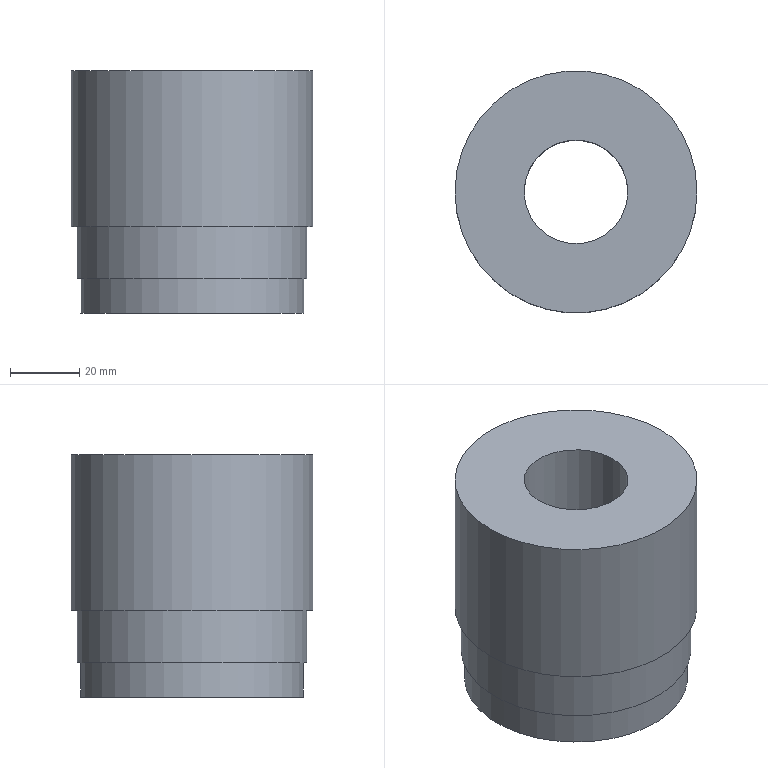Part | NX | features solid 2 | 1 solid | 8 faces | box 69.911 x 69.911 x 70 mm | volume 207947 mm3 | plane 4 | cylinder 4 | commonest cylinder face diameters 30 x1 64.492 x1 66.451 x1 69.911 x1
STEP:
#1=CARTESIAN_POINT('',(-46.774,-440.,-241.));
#2=VERTEX_POINT('',#1);
#3=CARTESIAN_POINT('',(-80.,-440.,-241.));
#4=DIRECTION('',(0.,0.,1.));
#5=DIRECTION('',(1.,0.,0.));
#6=AXIS2_PLACEMENT_3D('',#3,#4,#5);
#7=CIRCLE('',#6,33.226);
#8=EDGE_CURVE('',#2,#2,#7,.T.);
#9=ORIENTED_EDGE('',*,*,#8,.F.);
#10=EDGE_LOOP('',(#9));
#11=FACE_BOUND('',#10,.T.);
#12=CARTESIAN_POINT('',(-47.754,-440.,-241.));
#13=VERTEX_POINT('',#12);
#14=CARTESIAN_POINT('',(-80.,-440.,-241.));
#15=DIRECTION('',(0.,0.,1.));
#16=DIRECTION('',(1.,0.,0.));
#17=AXIS2_PLACEMENT_3D('',#14,#15,#16);
#18=CIRCLE('',#17,32.246);
#19=EDGE_CURVE('',#13,#13,#18,.F.);
#20=ORIENTED_EDGE('',*,*,#19,.F.);
#21=EDGE_LOOP('',(#20));
#22=FACE_BOUND('',#21,.T.);
#23=CARTESIAN_POINT('',(-80.,-440.,-241.));
#24=DIRECTION('',(0.,0.,-1.));
#25=DIRECTION('',(1.,0.,0.));
#26=AXIS2_PLACEMENT_3D('',#23,#24,#25);
#27=PLANE('',#26);
#28=ADVANCED_FACE('',(#11,#22),#27,.T.);
#29=CARTESIAN_POINT('',(-45.045,-440.,-226.));
#30=VERTEX_POINT('',#29);
#31=CARTESIAN_POINT('',(-80.,-440.,-226.));
#32=DIRECTION('',(0.,0.,1.));
#33=DIRECTION('',(1.,0.,0.));
#34=AXIS2_PLACEMENT_3D('',#31,#32,#33);
#35=CIRCLE('',#34,34.955);
#36=EDGE_CURVE('',#30,#30,#35,.T.);
#37=ORIENTED_EDGE('',*,*,#36,.F.);
#38=EDGE_LOOP('',(#37));
#39=FACE_BOUND('',#38,.T.);
#40=CARTESIAN_POINT('',(-46.774,-440.,-226.));
#41=VERTEX_POINT('',#40);
#42=CARTESIAN_POINT('',(-80.,-440.,-226.));
#43=DIRECTION('',(0.,0.,1.));
#44=DIRECTION('',(1.,0.,0.));
#45=AXIS2_PLACEMENT_3D('',#42,#43,#44);
#46=CIRCLE('',#45,33.226);
#47=EDGE_CURVE('',#41,#41,#46,.F.);
#48=ORIENTED_EDGE('',*,*,#47,.F.);
#49=EDGE_LOOP('',(#48));
#50=FACE_BOUND('',#49,.T.);
#51=CARTESIAN_POINT('',(-80.,-440.,-226.));
#52=DIRECTION('',(0.,0.,-1.));
#53=DIRECTION('',(1.,0.,0.));
#54=AXIS2_PLACEMENT_3D('',#51,#52,#53);
#55=PLANE('',#54);
#56=ADVANCED_FACE('',(#39,#50),#55,.T.);
#57=CARTESIAN_POINT('',(-65.,-440.,-181.));
#58=VERTEX_POINT('',#57);
#59=CARTESIAN_POINT('',(-80.,-440.,-181.));
#60=DIRECTION('',(0.,0.,1.));
#61=DIRECTION('',(1.,0.,0.));
#62=AXIS2_PLACEMENT_3D('',#59,#60,#61);
#63=CIRCLE('',#62,15.);
#64=EDGE_CURVE('',#58,#58,#63,.T.);
#65=ORIENTED_EDGE('',*,*,#64,.T.);
#66=EDGE_LOOP('',(#65));
#67=FACE_BOUND('',#66,.T.);
#68=CARTESIAN_POINT('',(-65.,-440.,-251.));
#69=VERTEX_POINT('',#68);
#70=CARTESIAN_POINT('',(-80.,-440.,-251.));
#71=DIRECTION('',(0.,0.,1.));
#72=DIRECTION('',(1.,0.,0.));
#73=AXIS2_PLACEMENT_3D('',#70,#71,#72);
#74=CIRCLE('',#73,15.);
#75=EDGE_CURVE('',#69,#69,#74,.T.);
#76=ORIENTED_EDGE('',*,*,#75,.F.);
#77=EDGE_LOOP('',(#76));
#78=FACE_BOUND('',#77,.T.);
#79=CARTESIAN_POINT('',(-80.,-440.,-226.));
#80=DIRECTION('',(0.,0.,1.));
#81=DIRECTION('',(-1.,0.,0.));
#82=AXIS2_PLACEMENT_3D('',#79,#80,#81);
#83=CYLINDRICAL_SURFACE('',#82,15.);
#84=ADVANCED_FACE('',(#67,#78),#83,.F.);
#85=ORIENTED_EDGE('',*,*,#36,.T.);
#86=EDGE_LOOP('',(#85));
#87=FACE_BOUND('',#86,.T.);
#88=CARTESIAN_POINT('',(-45.045,-440.,-181.));
#89=VERTEX_POINT('',#88);
#90=CARTESIAN_POINT('',(-80.,-440.,-181.));
#91=DIRECTION('',(0.,0.,1.));
#92=DIRECTION('',(1.,0.,0.));
#93=AXIS2_PLACEMENT_3D('',#90,#91,#92);
#94=CIRCLE('',#93,34.955);
#95=EDGE_CURVE('',#89,#89,#94,.T.);
#96=ORIENTED_EDGE('',*,*,#95,.F.);
#97=EDGE_LOOP('',(#96));
#98=FACE_BOUND('',#97,.T.);
#99=CARTESIAN_POINT('',(-80.,-440.,-226.));
#100=DIRECTION('',(0.,0.,1.));
#101=DIRECTION('',(-1.,0.,0.));
#102=AXIS2_PLACEMENT_3D('',#99,#100,#101);
#103=CYLINDRICAL_SURFACE('',#102,34.955);
#104=ADVANCED_FACE('',(#87,#98),#103,.T.);
#105=ORIENTED_EDGE('',*,*,#64,.F.);
#106=EDGE_LOOP('',(#105));
#107=FACE_BOUND('',#106,.T.);
#108=ORIENTED_EDGE('',*,*,#95,.T.);
#109=EDGE_LOOP('',(#108));
#110=FACE_BOUND('',#109,.T.);
#111=CARTESIAN_POINT('',(-80.,-440.,-181.));
#112=DIRECTION('',(0.,0.,-1.));
#113=DIRECTION('',(1.,0.,0.));
#114=AXIS2_PLACEMENT_3D('',#111,#112,#113);
#115=PLANE('',#114);
#116=ADVANCED_FACE('',(#107,#110),#115,.F.);
#117=ORIENTED_EDGE('',*,*,#47,.T.);
#118=EDGE_LOOP('',(#117));
#119=FACE_BOUND('',#118,.T.);
#120=ORIENTED_EDGE('',*,*,#8,.T.);
#121=EDGE_LOOP('',(#120));
#122=FACE_BOUND('',#121,.T.);
#123=CARTESIAN_POINT('',(-80.,-440.,-241.));
#124=DIRECTION('',(0.,0.,1.));
#125=DIRECTION('',(-1.,0.,0.));
#126=AXIS2_PLACEMENT_3D('',#123,#124,#125);
#127=CYLINDRICAL_SURFACE('',#126,33.226);
#128=ADVANCED_FACE('',(#119,#122),#127,.T.);
#129=ORIENTED_EDGE('',*,*,#19,.T.);
#130=EDGE_LOOP('',(#129));
#131=FACE_BOUND('',#130,.T.);
#132=CARTESIAN_POINT('',(-47.754,-440.,-251.));
#133=VERTEX_POINT('',#132);
#134=CARTESIAN_POINT('',(-80.,-440.,-251.));
#135=DIRECTION('',(0.,0.,1.));
#136=DIRECTION('',(1.,0.,0.));
#137=AXIS2_PLACEMENT_3D('',#134,#135,#136);
#138=CIRCLE('',#137,32.246);
#139=EDGE_CURVE('',#133,#133,#138,.T.);
#140=ORIENTED_EDGE('',*,*,#139,.T.);
#141=EDGE_LOOP('',(#140));
#142=FACE_BOUND('',#141,.T.);
#143=CARTESIAN_POINT('',(-80.,-440.,-251.));
#144=DIRECTION('',(0.,0.,1.));
#145=DIRECTION('',(-1.,0.,0.));
#146=AXIS2_PLACEMENT_3D('',#143,#144,#145);
#147=CYLINDRICAL_SURFACE('',#146,32.246);
#148=ADVANCED_FACE('',(#131,#142),#147,.T.);
#149=ORIENTED_EDGE('',*,*,#75,.T.);
#150=EDGE_LOOP('',(#149));
#151=FACE_BOUND('',#150,.T.);
#152=ORIENTED_EDGE('',*,*,#139,.F.);
#153=EDGE_LOOP('',(#152));
#154=FACE_BOUND('',#153,.T.);
#155=CARTESIAN_POINT('',(-80.,-440.,-251.));
#156=DIRECTION('',(0.,0.,-1.));
#157=DIRECTION('',(1.,0.,0.));
#158=AXIS2_PLACEMENT_3D('',#155,#156,#157);
#159=PLANE('',#158);
#160=ADVANCED_FACE('',(#151,#154),#159,.T.);
#161=CLOSED_SHELL('',(#28,#56,#84,#104,#116,#128,#148,#160));
#162=MANIFOLD_SOLID_BREP('',#161);
#163=(LENGTH_UNIT()NAMED_UNIT(*)SI_UNIT(.MILLI.,.METRE.));
#164=UNCERTAINTY_MEASURE_WITH_UNIT(LENGTH_MEASURE(0.00001),#163,'','');
#165=(NAMED_UNIT(*)PLANE_ANGLE_UNIT()SI_UNIT($,.RADIAN.));
#166=(NAMED_UNIT(*)SI_UNIT($,.STERADIAN.)SOLID_ANGLE_UNIT());
#167=(GEOMETRIC_REPRESENTATION_CONTEXT(3)GLOBAL_UNCERTAINTY_ASSIGNED_CONTEXT((#164))GLOBAL_UNIT_ASSIGNED_CONTEXT((#163,#165,#166))REPRESENTATION_CONTEXT('',''));
#168=ADVANCED_BREP_SHAPE_REPRESENTATION('',(#162),#167);